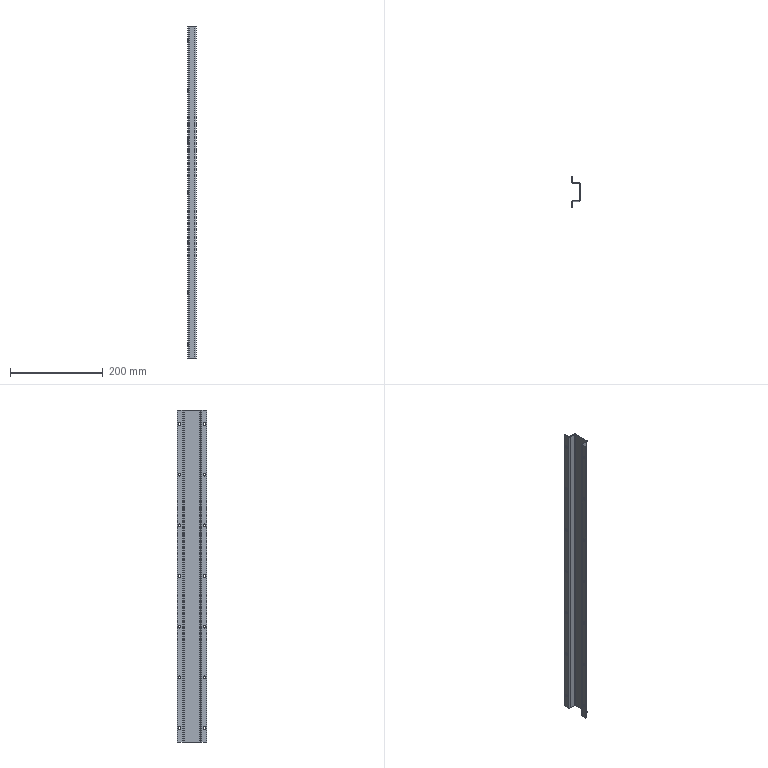Part | NX | features solid 2 | 1 solid | 50 faces | box 18.5 x 64 x 715 mm | volume 100368 mm3 | cylinder 36 | plane 14 | commonest cylinder face diameters 6 x32 3 x4